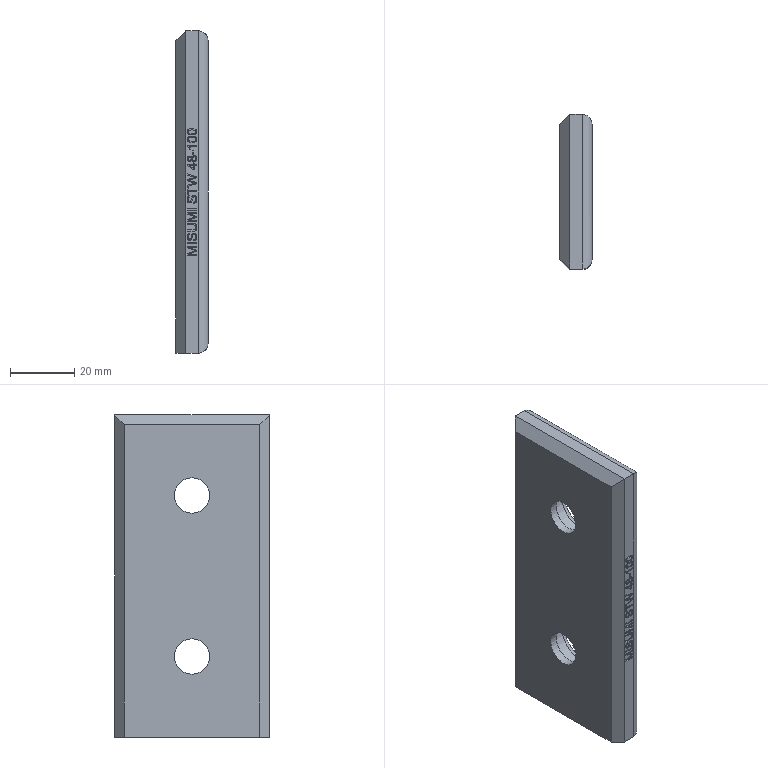Part | NX | features FD 2 | 1 solid | 153 faces | box 10 x 48 x 100 mm | volume 42152 mm3 | plane 106 | spline 37 | cylinder 8 | torus 2 | commonest cylinder face diameters 6 x4 11 x2 17.5 x2